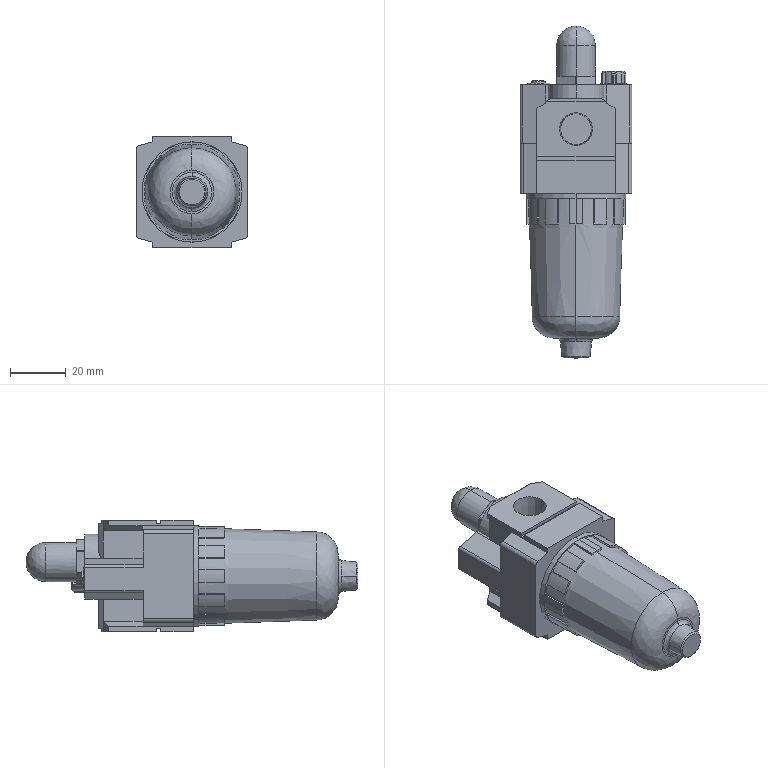Part | STEP file | 1 solid | 249 faces | box 40 x 119 x 40 mm | volume 93159 mm3 | plane 144 | cylinder 62 | cone 37 | spline 6 | commonest cylinder face diameters 35.5 x13 3.242 x8 8 x8 16 x7 2 x4 3 x4